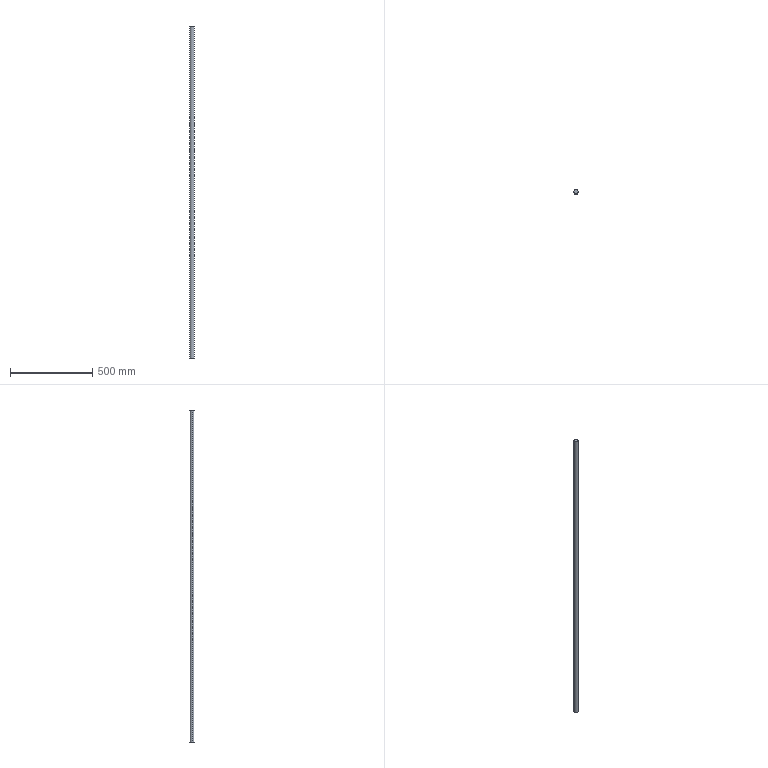Part | STEP file | 750038421 | 1 solid | 4 faces | box 25.4 x 25.4 x 2024 mm | volume 1025576 mm3 | cylinder 2 | plane 2 | commonest cylinder face diameters 25.4 x2
STEP:
#1=CARTESIAN_POINT('',(-12.7,0.,2024.));
#2=VERTEX_POINT('',#1);
#3=CARTESIAN_POINT('',(12.7,0.,2024.));
#4=VERTEX_POINT('',#3);
#5=CARTESIAN_POINT('',(0.,0.,2024.));
#6=DIRECTION('',(0.,0.,-1.));
#7=DIRECTION('',(-1.,0.,0.));
#8=AXIS2_PLACEMENT_3D('',#5,#6,#7);
#9=CIRCLE('',#8,12.7);
#10=EDGE_CURVE('',#2,#4,#9,.T.);
#11=ORIENTED_EDGE('',*,*,#10,.T.);
#12=CARTESIAN_POINT('',(12.7,0.,0.));
#13=VERTEX_POINT('',#12);
#14=CARTESIAN_POINT('',(12.7,0.,2024.));
#15=DIRECTION('',(0.,0.,-1.));
#16=VECTOR('',#15,1000.);
#17=LINE('',#14,#16);
#18=EDGE_CURVE('',#4,#13,#17,.T.);
#19=ORIENTED_EDGE('',*,*,#18,.T.);
#20=CARTESIAN_POINT('',(-12.7,0.,0.));
#21=VERTEX_POINT('',#20);
#22=CARTESIAN_POINT('',(0.,0.,0.));
#23=DIRECTION('',(0.,0.,1.));
#24=DIRECTION('',(-1.,0.,0.));
#25=AXIS2_PLACEMENT_3D('',#22,#23,#24);
#26=CIRCLE('',#25,12.7);
#27=EDGE_CURVE('',#13,#21,#26,.T.);
#28=ORIENTED_EDGE('',*,*,#27,.T.);
#29=CARTESIAN_POINT('',(-12.7,0.,2024.));
#30=DIRECTION('',(0.,0.,-1.));
#31=VECTOR('',#30,1000.);
#32=LINE('',#29,#31);
#33=EDGE_CURVE('',#2,#21,#32,.T.);
#34=ORIENTED_EDGE('',*,*,#33,.F.);
#35=EDGE_LOOP('',(#11,#19,#28,#34));
#36=FACE_OUTER_BOUND('',#35,.T.);
#37=CARTESIAN_POINT('',(0.,0.,2024.));
#38=DIRECTION('',(0.,0.,-1.));
#39=DIRECTION('',(-1.,0.,0.));
#40=AXIS2_PLACEMENT_3D('',#37,#38,#39);
#41=CYLINDRICAL_SURFACE('',#40,12.7);
#42=ADVANCED_FACE('',(#36),#41,.T.);
#43=ORIENTED_EDGE('',*,*,#18,.F.);
#44=CARTESIAN_POINT('',(0.,0.,2024.));
#45=DIRECTION('',(0.,0.,-1.));
#46=DIRECTION('',(-1.,0.,0.));
#47=AXIS2_PLACEMENT_3D('',#44,#45,#46);
#48=CIRCLE('',#47,12.7);
#49=EDGE_CURVE('',#4,#2,#48,.T.);
#50=ORIENTED_EDGE('',*,*,#49,.T.);
#51=ORIENTED_EDGE('',*,*,#33,.T.);
#52=CARTESIAN_POINT('',(0.,0.,0.));
#53=DIRECTION('',(0.,0.,1.));
#54=DIRECTION('',(-1.,0.,0.));
#55=AXIS2_PLACEMENT_3D('',#52,#53,#54);
#56=CIRCLE('',#55,12.7);
#57=EDGE_CURVE('',#21,#13,#56,.T.);
#58=ORIENTED_EDGE('',*,*,#57,.T.);
#59=EDGE_LOOP('',(#43,#50,#51,#58));
#60=FACE_OUTER_BOUND('',#59,.T.);
#61=CARTESIAN_POINT('',(0.,0.,2024.));
#62=DIRECTION('',(0.,0.,-1.));
#63=DIRECTION('',(-1.,0.,0.));
#64=AXIS2_PLACEMENT_3D('',#61,#62,#63);
#65=CYLINDRICAL_SURFACE('',#64,12.7);
#66=ADVANCED_FACE('',(#60),#65,.T.);
#67=ORIENTED_EDGE('',*,*,#57,.F.);
#68=ORIENTED_EDGE('',*,*,#27,.F.);
#69=EDGE_LOOP('',(#67,#68));
#70=FACE_OUTER_BOUND('',#69,.T.);
#71=CARTESIAN_POINT('',(0.,0.,0.));
#72=DIRECTION('',(0.,0.,1.));
#73=DIRECTION('',(1.,0.,0.));
#74=AXIS2_PLACEMENT_3D('',#71,#72,#73);
#75=PLANE('',#74);
#76=ADVANCED_FACE('',(#70),#75,.F.);
#77=ORIENTED_EDGE('',*,*,#10,.F.);
#78=ORIENTED_EDGE('',*,*,#49,.F.);
#79=EDGE_LOOP('',(#77,#78));
#80=FACE_OUTER_BOUND('',#79,.T.);
#81=CARTESIAN_POINT('',(0.,0.,2024.));
#82=DIRECTION('',(0.,0.,1.));
#83=DIRECTION('',(1.,0.,0.));
#84=AXIS2_PLACEMENT_3D('',#81,#82,#83);
#85=PLANE('',#84);
#86=ADVANCED_FACE('',(#80),#85,.T.);
#87=CLOSED_SHELL('',(#42,#66,#76,#86));
#88=MANIFOLD_SOLID_BREP('',#87);
#89=CARTESIAN_POINT('',(0.,0.,0.));
#90=DIRECTION('',(0.,0.,1.));
#91=DIRECTION('',(1.,0.,0.));
#92=AXIS2_PLACEMENT_3D('',#89,#90,#91);
#93=(LENGTH_UNIT()NAMED_UNIT(*)SI_UNIT(.MILLI.,.METRE.));
#94=UNCERTAINTY_MEASURE_WITH_UNIT(LENGTH_MEASURE(0.00001),#93,'','');
#95=(NAMED_UNIT(*)PLANE_ANGLE_UNIT()SI_UNIT($,.RADIAN.));
#96=(NAMED_UNIT(*)SI_UNIT($,.STERADIAN.)SOLID_ANGLE_UNIT());
#97=(GEOMETRIC_REPRESENTATION_CONTEXT(3)GLOBAL_UNCERTAINTY_ASSIGNED_CONTEXT((#94))GLOBAL_UNIT_ASSIGNED_CONTEXT((#93,#95,#96))REPRESENTATION_CONTEXT('',''));
#98=ADVANCED_BREP_SHAPE_REPRESENTATION('',(#88,#92),#97);